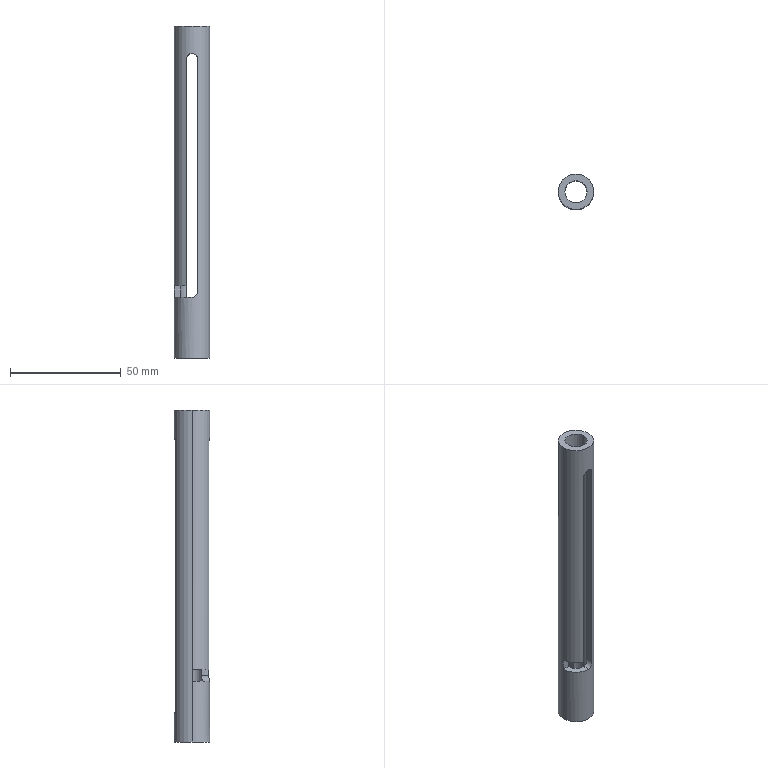Part | STEP file | PN_0102 Mount electronic clip sensor A | 1 solid | 21 faces | box 16 x 16 x 150 mm | volume 14386 mm3 | plane 12 | cylinder 9 | commonest cylinder face diameters 5.2 x5 10 x2 16 x2